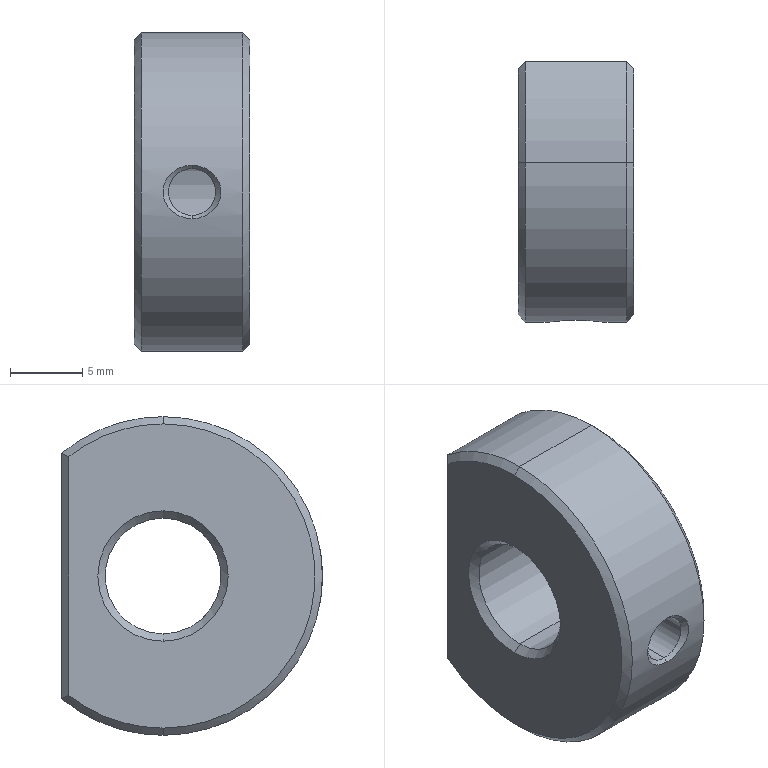Part | STEP file | 0246_Z_003_PSDSN8_1 | 1 solid | 41 faces | box 8 x 18 x 22 mm | volume 2101 mm3 | cone 22 | cylinder 14 | plane 5 | commonest cylinder face diameters 2.459 x4 4 x3 22 x3 3.242 x2 8 x2